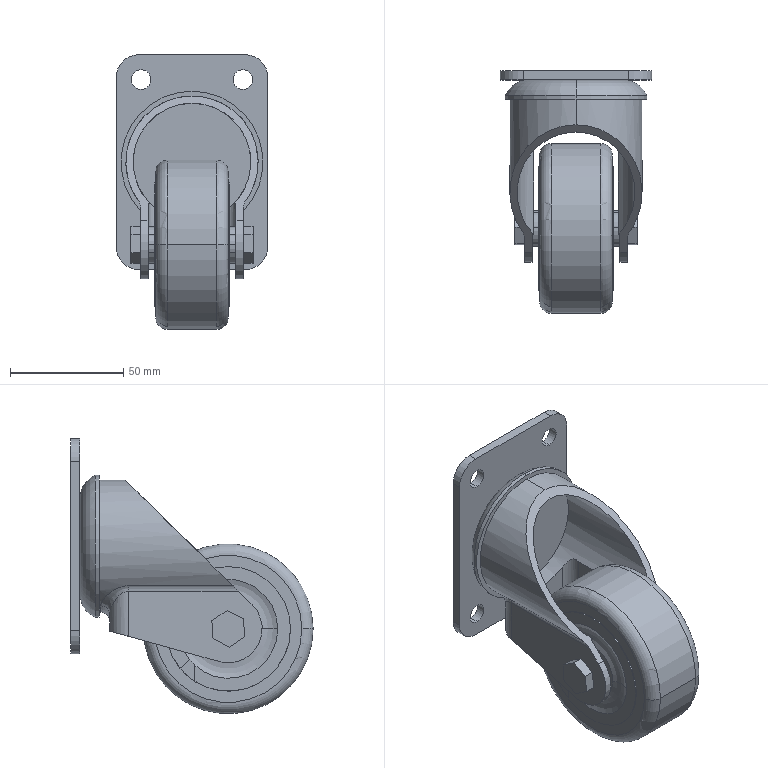Part | SolidWorks | features Cut 6, Boss 5, Fillet 2, Revolution 2, Extrusion 1 | 2 solids | 103 faces | box 67 x 107 x 121.5 mm | volume 222631 mm3 | plane 52 | cylinder 38 | torus 11 | spline 2 | commonest cylinder face diameters 8.636 x8 15.875 x4 20.32 x4 30 x4 55 x4 7.938 x2